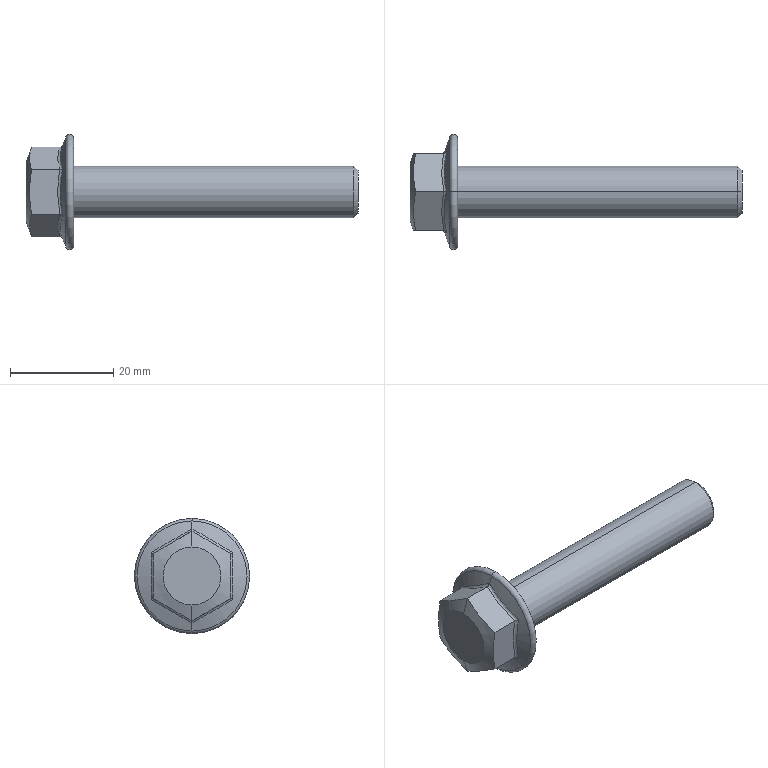Part | SolidWorks | features Fillet 2, RevCut 2, Boss 1, Chamfer 1, Extrusion 1, LPattern 1, Revolution 1 | 1 solid | 25 faces | box 64.2 x 22.3 x 22.3 mm | volume 6417 mm3 | plane 9 | cone 6 | spline 6 | torus 2 | cylinder 2 | commonest cylinder face diameters 10 x2
STEP:
#1=CARTESIAN_POINT('',(64.2,0.,-4.188));
#2=VERTEX_POINT('',#1);
#3=CARTESIAN_POINT('',(64.2,0.,4.188));
#4=VERTEX_POINT('',#3);
#5=CARTESIAN_POINT('',(64.2,0.,0.));
#6=DIRECTION('',(1.,0.,0.));
#7=DIRECTION('',(0.,0.,-1.));
#8=AXIS2_PLACEMENT_3D('',#5,#6,#7);
#9=CIRCLE('',#8,4.188);
#10=EDGE_CURVE('',#2,#4,#9,.T.);
#11=ORIENTED_EDGE('',*,*,#10,.F.);
#12=CARTESIAN_POINT('',(63.388,0.,-5.));
#13=VERTEX_POINT('',#12);
#14=CARTESIAN_POINT('',(64.2,0.,-4.188));
#15=DIRECTION('',(-0.7071,0.,-0.7071));
#16=VECTOR('',#15,1000.);
#17=LINE('',#14,#16);
#18=EDGE_CURVE('',#2,#13,#17,.T.);
#19=ORIENTED_EDGE('',*,*,#18,.T.);
#20=CARTESIAN_POINT('',(63.388,0.,5.));
#21=VERTEX_POINT('',#20);
#22=CARTESIAN_POINT('',(63.388,0.,0.));
#23=DIRECTION('',(-1.,0.,0.));
#24=DIRECTION('',(0.,0.,-1.));
#25=AXIS2_PLACEMENT_3D('',#22,#23,#24);
#26=CIRCLE('',#25,5.);
#27=EDGE_CURVE('',#21,#13,#26,.T.);
#28=ORIENTED_EDGE('',*,*,#27,.F.);
#29=CARTESIAN_POINT('',(64.2,0.,4.188));
#30=DIRECTION('',(-0.7071,0.,0.7071));
#31=VECTOR('',#30,1000.);
#32=LINE('',#29,#31);
#33=EDGE_CURVE('',#4,#21,#32,.T.);
#34=ORIENTED_EDGE('',*,*,#33,.F.);
#35=EDGE_LOOP('',(#11,#19,#28,#34));
#36=FACE_OUTER_BOUND('',#35,.T.);
#37=CARTESIAN_POINT('',(64.2,0.,0.));
#38=DIRECTION('',(-1.,0.,0.));
#39=DIRECTION('',(0.,0.,1.));
#40=AXIS2_PLACEMENT_3D('',#37,#38,#39);
#41=CONICAL_SURFACE('',#40,4.188,0.7854);
#42=ADVANCED_FACE('',(#36),#41,.T.);
#43=CARTESIAN_POINT('',(0.,0.,5.6));
#44=VERTEX_POINT('',#43);
#45=CARTESIAN_POINT('',(0.,0.,-5.6));
#46=VERTEX_POINT('',#45);
#47=CARTESIAN_POINT('',(0.,0.,0.));
#48=DIRECTION('',(-1.,0.,0.));
#49=DIRECTION('',(0.,0.,1.));
#50=AXIS2_PLACEMENT_3D('',#47,#48,#49);
#51=CIRCLE('',#50,5.6);
#52=EDGE_CURVE('',#44,#46,#51,.T.);
#53=ORIENTED_EDGE('',*,*,#52,.F.);
#54=CARTESIAN_POINT('',(1.114,0.,8.66));
#55=VERTEX_POINT('',#54);
#56=CARTESIAN_POINT('',(0.,0.,5.6));
#57=DIRECTION('',(0.342,0.,0.9397));
#58=VECTOR('',#57,1000.);
#59=LINE('',#56,#58);
#60=EDGE_CURVE('',#44,#55,#59,.T.);
#61=ORIENTED_EDGE('',*,*,#60,.T.);
#62=CARTESIAN_POINT('',(1.114,7.5,4.33));
#63=VERTEX_POINT('',#62);
#64=CARTESIAN_POINT('',(1.114,0.,8.66));
#65=CARTESIAN_POINT('',(0.9825,0.625,8.299));
#66=CARTESIAN_POINT('',(0.8759,1.25,7.939));
#67=CARTESIAN_POINT('',(0.7302,2.5,7.217));
#68=CARTESIAN_POINT('',(0.6529,3.75,6.495));
#69=CARTESIAN_POINT('',(0.7302,5.,5.774));
#70=CARTESIAN_POINT('',(0.8759,6.25,5.052));
#71=CARTESIAN_POINT('',(0.9825,6.875,4.691));
#72=CARTESIAN_POINT('',(1.114,7.5,4.33));
#73=B_SPLINE_CURVE_WITH_KNOTS('',3,(#64,#65,#66,#67,#68,#69,#70,#71,#72),.UNSPECIFIED.,.F.,.F.,(4,2,1,2,4),(0.000000231,0.002165,0.00433,0.006495,0.00866),.UNSPECIFIED.);
#74=EDGE_CURVE('',#55,#63,#73,.T.);
#75=ORIENTED_EDGE('',*,*,#74,.T.);
#76=CARTESIAN_POINT('',(1.114,7.5,-4.33));
#77=VERTEX_POINT('',#76);
#78=CARTESIAN_POINT('',(1.114,7.5,4.33));
#79=CARTESIAN_POINT('',(0.983,7.5,3.611));
#80=CARTESIAN_POINT('',(0.8765,7.5,2.891));
#81=CARTESIAN_POINT('',(0.7307,7.5,1.45));
#82=CARTESIAN_POINT('',(0.6918,7.5,0.7288));
#83=CARTESIAN_POINT('',(0.6913,7.5,-0.7155));
#84=CARTESIAN_POINT('',(0.7298,7.5,-1.439));
#85=CARTESIAN_POINT('',(0.8757,7.5,-2.886));
#86=CARTESIAN_POINT('',(0.9832,7.5,-3.612));
#87=CARTESIAN_POINT('',(1.114,7.5,-4.33));
#88=B_SPLINE_CURVE_WITH_KNOTS('',3,(#78,#79,#80,#81,#82,#83,#84,#85,#86,#87),.UNSPECIFIED.,.F.,.F.,(4,2,2,2,4),(0.01595,0.01813,0.02031,0.02249,0.02467),.UNSPECIFIED.);
#89=EDGE_CURVE('',#63,#77,#88,.T.);
#90=ORIENTED_EDGE('',*,*,#89,.T.);
#91=CARTESIAN_POINT('',(1.114,0.,-8.66));
#92=VERTEX_POINT('',#91);
#93=CARTESIAN_POINT('',(1.114,7.5,-4.33));
#94=CARTESIAN_POINT('',(0.9825,6.875,-4.691));
#95=CARTESIAN_POINT('',(0.8759,6.25,-5.052));
#96=CARTESIAN_POINT('',(0.7302,5.,-5.774));
#97=CARTESIAN_POINT('',(0.6529,3.75,-6.495));
#98=CARTESIAN_POINT('',(0.7302,2.5,-7.217));
#99=CARTESIAN_POINT('',(0.8759,1.25,-7.939));
#100=CARTESIAN_POINT('',(0.9825,0.625,-8.299));
#101=CARTESIAN_POINT('',(1.114,0.,-8.66));
#102=B_SPLINE_CURVE_WITH_KNOTS('',3,(#93,#94,#95,#96,#97,#98,#99,#100,#101),.UNSPECIFIED.,.F.,.F.,(4,2,1,2,4),(0.000000231,0.002165,0.00433,0.006495,0.00866),.UNSPECIFIED.);
#103=EDGE_CURVE('',#77,#92,#102,.T.);
#104=ORIENTED_EDGE('',*,*,#103,.T.);
#105=CARTESIAN_POINT('',(0.,0.,-5.6));
#106=DIRECTION('',(0.342,0.,-0.9397));
#107=VECTOR('',#106,1000.);
#108=LINE('',#105,#107);
#109=EDGE_CURVE('',#46,#92,#108,.T.);
#110=ORIENTED_EDGE('',*,*,#109,.F.);
#111=EDGE_LOOP('',(#53,#61,#75,#90,#104,#110));
#112=FACE_OUTER_BOUND('',#111,.T.);
#113=CARTESIAN_POINT('',(0.,0.,0.));
#114=DIRECTION('',(1.,0.,0.));
#115=DIRECTION('',(0.,0.,-1.));
#116=AXIS2_PLACEMENT_3D('',#113,#114,#115);
#117=CONICAL_SURFACE('',#116,5.6,1.222);
#118=ADVANCED_FACE('',(#112),#117,.T.);
#119=CARTESIAN_POINT('',(7.7,0.,-10.641));
#120=VERTEX_POINT('',#119);
#121=CARTESIAN_POINT('',(7.7,0.,10.641));
#122=VERTEX_POINT('',#121);
#123=CARTESIAN_POINT('',(7.7,0.,0.));
#124=DIRECTION('',(1.,0.,0.));
#125=DIRECTION('',(0.,0.,-1.));
#126=AXIS2_PLACEMENT_3D('',#123,#124,#125);
#127=CIRCLE('',#126,10.641);
#128=EDGE_CURVE('',#120,#122,#127,.T.);
#129=ORIENTED_EDGE('',*,*,#128,.T.);
#130=CARTESIAN_POINT('',(9.2,0.,10.377));
#131=VERTEX_POINT('',#130);
#132=CARTESIAN_POINT('',(8.427,0.,10.377));
#133=DIRECTION('',(0.,1.,0.));
#134=DIRECTION('',(0.,0.,1.));
#135=AXIS2_PLACEMENT_3D('',#132,#133,#134);
#136=CIRCLE('',#135,0.7733);
#137=EDGE_CURVE('',#122,#131,#136,.T.);
#138=ORIENTED_EDGE('',*,*,#137,.T.);
#139=CARTESIAN_POINT('',(9.2,0.,-10.377));
#140=VERTEX_POINT('',#139);
#141=CARTESIAN_POINT('',(9.2,0.,0.));
#142=DIRECTION('',(1.,0.,0.));
#143=DIRECTION('',(0.,0.,-1.));
#144=AXIS2_PLACEMENT_3D('',#141,#142,#143);
#145=CIRCLE('',#144,10.377);
#146=EDGE_CURVE('',#140,#131,#145,.T.);
#147=ORIENTED_EDGE('',*,*,#146,.F.);
#148=CARTESIAN_POINT('',(8.427,0.,-10.377));
#149=DIRECTION('',(0.,-1.,0.));
#150=DIRECTION('',(0.,0.,-1.));
#151=AXIS2_PLACEMENT_3D('',#148,#149,#150);
#152=CIRCLE('',#151,0.7733);
#153=EDGE_CURVE('',#120,#140,#152,.T.);
#154=ORIENTED_EDGE('',*,*,#153,.F.);
#155=EDGE_LOOP('',(#129,#138,#147,#154));
#156=FACE_OUTER_BOUND('',#155,.T.);
#157=CARTESIAN_POINT('',(8.427,0.,0.));
#158=DIRECTION('',(1.,0.,0.));
#159=DIRECTION('',(0.,0.,-1.));
#160=AXIS2_PLACEMENT_3D('',#157,#158,#159);
#161=TOROIDAL_SURFACE('',#160,10.377,0.7733);
#162=ADVANCED_FACE('',(#156),#161,.T.);
#163=CARTESIAN_POINT('',(7.156,7.922,4.574));
#164=VERTEX_POINT('',#163);
#165=CARTESIAN_POINT('',(7.156,0.,9.148));
#166=VERTEX_POINT('',#165);
#167=CARTESIAN_POINT('',(7.156,7.922,4.574));
#168=CARTESIAN_POINT('',(7.017,7.265,4.945));
#169=CARTESIAN_POINT('',(6.902,6.605,5.318));
#170=CARTESIAN_POINT('',(6.744,5.282,6.07));
#171=CARTESIAN_POINT('',(6.701,4.619,6.45));
#172=CARTESIAN_POINT('',(6.7,3.287,7.218));
#173=CARTESIAN_POINT('',(6.743,2.624,7.605));
#174=CARTESIAN_POINT('',(6.901,1.305,8.378));
#175=CARTESIAN_POINT('',(7.017,0.6509,8.764));
#176=CARTESIAN_POINT('',(7.156,0.,9.148));
#177=B_SPLINE_CURVE_WITH_KNOTS('',3,(#167,#168,#169,#170,#171,#172,#173,#174,#175,#176),.UNSPECIFIED.,.F.,.F.,(4,2,2,2,4),(0.,0.002295,0.004591,0.006886,0.009181),.UNSPECIFIED.);
#178=EDGE_CURVE('',#164,#166,#177,.T.);
#179=ORIENTED_EDGE('',*,*,#178,.T.);
#180=CARTESIAN_POINT('',(7.7,0.,10.641));
#181=DIRECTION('',(0.342,0.,0.9397));
#182=VECTOR('',#181,1000.);
#183=LINE('',#180,#182);
#184=EDGE_CURVE('',#166,#122,#183,.T.);
#185=ORIENTED_EDGE('',*,*,#184,.T.);
#186=ORIENTED_EDGE('',*,*,#128,.F.);
#187=CARTESIAN_POINT('',(7.156,0.,-9.148));
#188=VERTEX_POINT('',#187);
#189=CARTESIAN_POINT('',(7.7,0.,-10.641));
#190=DIRECTION('',(0.342,0.,-0.9397));
#191=VECTOR('',#190,1000.);
#192=LINE('',#189,#191);
#193=EDGE_CURVE('',#188,#120,#192,.T.);
#194=ORIENTED_EDGE('',*,*,#193,.F.);
#195=CARTESIAN_POINT('',(7.156,7.922,-4.574));
#196=VERTEX_POINT('',#195);
#197=CARTESIAN_POINT('',(7.156,0.,-9.148));
#198=CARTESIAN_POINT('',(7.017,0.6501,-8.764));
#199=CARTESIAN_POINT('',(6.902,1.303,-8.379));
#200=CARTESIAN_POINT('',(6.744,2.616,-7.61));
#201=CARTESIAN_POINT('',(6.701,3.276,-7.225));
#202=CARTESIAN_POINT('',(6.7,4.608,-6.456));
#203=CARTESIAN_POINT('',(6.743,5.274,-6.075));
#204=CARTESIAN_POINT('',(6.901,6.603,-5.319));
#205=CARTESIAN_POINT('',(7.017,7.264,-4.945));
#206=CARTESIAN_POINT('',(7.156,7.922,-4.574));
#207=B_SPLINE_CURVE_WITH_KNOTS('',3,(#197,#198,#199,#200,#201,#202,#203,#204,#205,#206),.UNSPECIFIED.,.F.,.F.,(4,2,2,2,4),(0.,0.002295,0.004591,0.006886,0.009181),.UNSPECIFIED.);
#208=EDGE_CURVE('',#188,#196,#207,.T.);
#209=ORIENTED_EDGE('',*,*,#208,.T.);
#210=CARTESIAN_POINT('',(7.156,7.922,-4.574));
#211=CARTESIAN_POINT('',(7.017,7.915,-3.819));
#212=CARTESIAN_POINT('',(6.902,7.908,-3.062));
#213=CARTESIAN_POINT('',(6.744,7.898,-1.54));
#214=CARTESIAN_POINT('',(6.701,7.895,-0.7751));
#215=CARTESIAN_POINT('',(6.7,7.895,0.7626));
#216=CARTESIAN_POINT('',(6.743,7.898,1.53));
#217=CARTESIAN_POINT('',(6.901,7.908,3.059));
#218=CARTESIAN_POINT('',(7.017,7.915,3.818));
#219=CARTESIAN_POINT('',(7.156,7.922,4.574));
#220=B_SPLINE_CURVE_WITH_KNOTS('',3,(#210,#211,#212,#213,#214,#215,#216,#217,#218,#219),.UNSPECIFIED.,.F.,.F.,(4,2,2,2,4),(0.,0.002295,0.00459,0.006886,0.009181),.UNSPECIFIED.);
#221=EDGE_CURVE('',#196,#164,#220,.T.);
#222=ORIENTED_EDGE('',*,*,#221,.T.);
#223=EDGE_LOOP('',(#179,#185,#186,#194,#209,#222));
#224=FACE_OUTER_BOUND('',#223,.T.);
#225=CARTESIAN_POINT('',(7.7,0.,0.));
#226=DIRECTION('',(1.,0.,0.));
#227=DIRECTION('',(0.,0.,-1.));
#228=AXIS2_PLACEMENT_3D('',#225,#226,#227);
#229=CONICAL_SURFACE('',#228,10.641,1.222);
#230=ADVANCED_FACE('',(#224),#229,.T.);
#231=ORIENTED_EDGE('',*,*,#27,.T.);
#232=CARTESIAN_POINT('',(9.2,0.,-5.));
#233=VERTEX_POINT('',#232);
#234=CARTESIAN_POINT('',(64.2,0.,-5.));
#235=DIRECTION('',(-1.,0.,0.));
#236=VECTOR('',#235,1000.);
#237=LINE('',#234,#236);
#238=EDGE_CURVE('',#13,#233,#237,.T.);
#239=ORIENTED_EDGE('',*,*,#238,.T.);
#240=CARTESIAN_POINT('',(9.2,0.,5.));
#241=VERTEX_POINT('',#240);
#242=CARTESIAN_POINT('',(9.2,0.,0.));
#243=DIRECTION('',(1.,0.,0.));
#244=DIRECTION('',(0.,0.,-1.));
#245=AXIS2_PLACEMENT_3D('',#242,#243,#244);
#246=CIRCLE('',#245,5.);
#247=EDGE_CURVE('',#233,#241,#246,.T.);
#248=ORIENTED_EDGE('',*,*,#247,.T.);
#249=CARTESIAN_POINT('',(64.2,0.,5.));
#250=DIRECTION('',(-1.,0.,0.));
#251=VECTOR('',#250,1000.);
#252=LINE('',#249,#251);
#253=EDGE_CURVE('',#21,#241,#252,.T.);
#254=ORIENTED_EDGE('',*,*,#253,.F.);
#255=EDGE_LOOP('',(#231,#239,#248,#254));
#256=FACE_OUTER_BOUND('',#255,.T.);
#257=CARTESIAN_POINT('',(64.2,0.,0.));
#258=DIRECTION('',(-1.,0.,0.));
#259=DIRECTION('',(0.,0.,1.));
#260=AXIS2_PLACEMENT_3D('',#257,#258,#259);
#261=CYLINDRICAL_SURFACE('',#260,5.);
#262=ADVANCED_FACE('',(#256),#261,.T.);
#263=CARTESIAN_POINT('',(9.2,0.,0.));
#264=DIRECTION('',(1.,0.,0.));
#265=DIRECTION('',(0.,0.,-1.));
#266=AXIS2_PLACEMENT_3D('',#263,#264,#265);
#267=CIRCLE('',#266,5.);
#268=EDGE_CURVE('',#241,#233,#267,.T.);
#269=ORIENTED_EDGE('',*,*,#268,.F.);
#270=ORIENTED_EDGE('',*,*,#247,.F.);
#271=EDGE_LOOP('',(#269,#270));
#272=FACE_BOUND('',#271,.T.);
#273=ORIENTED_EDGE('',*,*,#146,.T.);
#274=CARTESIAN_POINT('',(9.2,0.,0.));
#275=DIRECTION('',(1.,0.,0.));
#276=DIRECTION('',(0.,0.,-1.));
#277=AXIS2_PLACEMENT_3D('',#274,#275,#276);
#278=CIRCLE('',#277,10.377);
#279=EDGE_CURVE('',#131,#140,#278,.T.);
#280=ORIENTED_EDGE('',*,*,#279,.T.);
#281=EDGE_LOOP('',(#273,#280));
#282=FACE_OUTER_BOUND('',#281,.T.);
#283=CARTESIAN_POINT('',(9.2,7.5,-12.99));
#284=DIRECTION('',(1.,0.,0.));
#285=DIRECTION('',(0.,0.,-1.));
#286=AXIS2_PLACEMENT_3D('',#283,#284,#285);
#287=PLANE('',#286);
#288=ADVANCED_FACE('',(#272,#282),#287,.T.);
#289=ORIENTED_EDGE('',*,*,#238,.F.);
#290=CARTESIAN_POINT('',(63.388,0.,0.));
#291=DIRECTION('',(-1.,0.,0.));
#292=DIRECTION('',(0.,0.,-1.));
#293=AXIS2_PLACEMENT_3D('',#290,#291,#292);
#294=CIRCLE('',#293,5.);
#295=EDGE_CURVE('',#13,#21,#294,.T.);
#296=ORIENTED_EDGE('',*,*,#295,.T.);
#297=ORIENTED_EDGE('',*,*,#253,.T.);
#298=ORIENTED_EDGE('',*,*,#268,.T.);
#299=EDGE_LOOP('',(#289,#296,#297,#298));
#300=FACE_OUTER_BOUND('',#299,.T.);
#301=CARTESIAN_POINT('',(64.2,0.,0.));
#302=DIRECTION('',(-1.,0.,0.));
#303=DIRECTION('',(0.,0.,1.));
#304=AXIS2_PLACEMENT_3D('',#301,#302,#303);
#305=CYLINDRICAL_SURFACE('',#304,5.);
#306=ADVANCED_FACE('',(#300),#305,.T.);
#307=CARTESIAN_POINT('',(64.2,0.,0.));
#308=DIRECTION('',(1.,0.,0.));
#309=DIRECTION('',(0.,0.,-1.));
#310=AXIS2_PLACEMENT_3D('',#307,#308,#309);
#311=CIRCLE('',#310,4.188);
#312=EDGE_CURVE('',#4,#2,#311,.T.);
#313=ORIENTED_EDGE('',*,*,#312,.T.);
#314=ORIENTED_EDGE('',*,*,#10,.T.);
#315=EDGE_LOOP('',(#313,#314));
#316=FACE_OUTER_BOUND('',#315,.T.);
#317=CARTESIAN_POINT('',(64.2,0.,0.));
#318=DIRECTION('',(1.,0.,0.));
#319=DIRECTION('',(0.,0.,-1.));
#320=AXIS2_PLACEMENT_3D('',#317,#318,#319);
#321=PLANE('',#320);
#322=ADVANCED_FACE('',(#316),#321,.T.);
#323=ORIENTED_EDGE('',*,*,#184,.F.);
#324=CARTESIAN_POINT('',(7.156,-7.922,4.574));
#325=VERTEX_POINT('',#324);
#326=CARTESIAN_POINT('',(7.156,0.,9.148));
#327=CARTESIAN_POINT('',(7.017,-0.6501,8.764));
#328=CARTESIAN_POINT('',(6.902,-1.303,8.379));
#329=CARTESIAN_POINT('',(6.744,-2.616,7.61));
#330=CARTESIAN_POINT('',(6.701,-3.276,7.225));
#331=CARTESIAN_POINT('',(6.7,-4.608,6.456));
#332=CARTESIAN_POINT('',(6.743,-5.274,6.075));
#333=CARTESIAN_POINT('',(6.901,-6.603,5.319));
#334=CARTESIAN_POINT('',(7.017,-7.264,4.945));
#335=CARTESIAN_POINT('',(7.156,-7.922,4.574));
#336=B_SPLINE_CURVE_WITH_KNOTS('',3,(#326,#327,#328,#329,#330,#331,#332,#333,#334,#335),.UNSPECIFIED.,.F.,.F.,(4,2,2,2,4),(0.,0.002295,0.004591,0.006886,0.009181),.UNSPECIFIED.);
#337=EDGE_CURVE('',#166,#325,#336,.T.);
#338=ORIENTED_EDGE('',*,*,#337,.T.);
#339=CARTESIAN_POINT('',(7.156,-7.922,-4.574));
#340=VERTEX_POINT('',#339);
#341=CARTESIAN_POINT('',(7.156,-7.922,4.574));
#342=CARTESIAN_POINT('',(7.017,-7.915,3.819));
#343=CARTESIAN_POINT('',(6.902,-7.908,3.062));
#344=CARTESIAN_POINT('',(6.744,-7.898,1.54));
#345=CARTESIAN_POINT('',(6.701,-7.895,0.775));
#346=CARTESIAN_POINT('',(6.7,-7.895,-0.7627));
#347=CARTESIAN_POINT('',(6.743,-7.898,-1.53));
#348=CARTESIAN_POINT('',(6.901,-7.908,-3.059));
#349=CARTESIAN_POINT('',(7.017,-7.915,-3.818));
#350=CARTESIAN_POINT('',(7.156,-7.922,-4.574));
#351=B_SPLINE_CURVE_WITH_KNOTS('',3,(#341,#342,#343,#344,#345,#346,#347,#348,#349,#350),.UNSPECIFIED.,.F.,.F.,(4,2,2,2,4),(0.,0.002295,0.004591,0.006886,0.009181),.UNSPECIFIED.);
#352=EDGE_CURVE('',#325,#340,#351,.T.);
#353=ORIENTED_EDGE('',*,*,#352,.T.);
#354=CARTESIAN_POINT('',(7.156,-7.922,-4.574));
#355=CARTESIAN_POINT('',(7.017,-7.265,-4.945));
#356=CARTESIAN_POINT('',(6.902,-6.605,-5.318));
#357=CARTESIAN_POINT('',(6.744,-5.282,-6.07));
#358=CARTESIAN_POINT('',(6.701,-4.619,-6.45));
#359=CARTESIAN_POINT('',(6.7,-3.287,-7.218));
#360=CARTESIAN_POINT('',(6.743,-2.624,-7.605));
#361=CARTESIAN_POINT('',(6.901,-1.305,-8.378));
#362=CARTESIAN_POINT('',(7.017,-0.6509,-8.764));
#363=CARTESIAN_POINT('',(7.156,0.,-9.148));
#364=B_SPLINE_CURVE_WITH_KNOTS('',3,(#354,#355,#356,#357,#358,#359,#360,#361,#362,#363),.UNSPECIFIED.,.F.,.F.,(4,2,2,2,4),(0.,0.002295,0.004591,0.006886,0.009181),.UNSPECIFIED.);
#365=EDGE_CURVE('',#340,#188,#364,.T.);
#366=ORIENTED_EDGE('',*,*,#365,.T.);
#367=ORIENTED_EDGE('',*,*,#193,.T.);
#368=CARTESIAN_POINT('',(7.7,0.,0.));
#369=DIRECTION('',(1.,0.,0.));
#370=DIRECTION('',(0.,0.,-1.));
#371=AXIS2_PLACEMENT_3D('',#368,#369,#370);
#372=CIRCLE('',#371,10.641);
#373=EDGE_CURVE('',#122,#120,#372,.T.);
#374=ORIENTED_EDGE('',*,*,#373,.F.);
#375=EDGE_LOOP('',(#323,#338,#353,#366,#367,#374));
#376=FACE_OUTER_BOUND('',#375,.T.);
#377=CARTESIAN_POINT('',(7.7,0.,0.));
#378=DIRECTION('',(1.,0.,0.));
#379=DIRECTION('',(0.,0.,-1.));
#380=AXIS2_PLACEMENT_3D('',#377,#378,#379);
#381=CONICAL_SURFACE('',#380,10.641,1.222);
#382=ADVANCED_FACE('',(#376),#381,.T.);
#383=ORIENTED_EDGE('',*,*,#137,.F.);
#384=ORIENTED_EDGE('',*,*,#373,.T.);
#385=ORIENTED_EDGE('',*,*,#153,.T.);
#386=ORIENTED_EDGE('',*,*,#279,.F.);
#387=EDGE_LOOP('',(#383,#384,#385,#386));
#388=FACE_OUTER_BOUND('',#387,.T.);
#389=CARTESIAN_POINT('',(8.427,0.,0.));
#390=DIRECTION('',(1.,0.,0.));
#391=DIRECTION('',(0.,0.,-1.));
#392=AXIS2_PLACEMENT_3D('',#389,#390,#391);
#393=TOROIDAL_SURFACE('',#392,10.377,0.7733);
#394=ADVANCED_FACE('',(#388),#393,.T.);
#395=CARTESIAN_POINT('',(0.,0.,0.));
#396=DIRECTION('',(-1.,0.,0.));
#397=DIRECTION('',(0.,0.,1.));
#398=AXIS2_PLACEMENT_3D('',#395,#396,#397);
#399=CIRCLE('',#398,5.6);
#400=EDGE_CURVE('',#46,#44,#399,.T.);
#401=ORIENTED_EDGE('',*,*,#400,.T.);
#402=ORIENTED_EDGE('',*,*,#52,.T.);
#403=EDGE_LOOP('',(#401,#402));
#404=FACE_OUTER_BOUND('',#403,.T.);
#405=CARTESIAN_POINT('',(0.,7.5,-12.99));
#406=DIRECTION('',(1.,0.,0.));
#407=DIRECTION('',(0.,0.,-1.));
#408=AXIS2_PLACEMENT_3D('',#405,#406,#407);
#409=PLANE('',#408);
#410=ADVANCED_FACE('',(#404),#409,.F.);
#411=ORIENTED_EDGE('',*,*,#60,.F.);
#412=ORIENTED_EDGE('',*,*,#400,.F.);
#413=ORIENTED_EDGE('',*,*,#109,.T.);
#414=CARTESIAN_POINT('',(1.114,-7.5,-4.33));
#415=VERTEX_POINT('',#414);
#416=CARTESIAN_POINT('',(1.114,0.,-8.66));
#417=CARTESIAN_POINT('',(0.9825,-0.625,-8.299));
#418=CARTESIAN_POINT('',(0.8759,-1.25,-7.939));
#419=CARTESIAN_POINT('',(0.7302,-2.5,-7.217));
#420=CARTESIAN_POINT('',(0.6529,-3.75,-6.495));
#421=CARTESIAN_POINT('',(0.7302,-5.,-5.774));
#422=CARTESIAN_POINT('',(0.8759,-6.25,-5.052));
#423=CARTESIAN_POINT('',(0.9825,-6.875,-4.691));
#424=CARTESIAN_POINT('',(1.114,-7.5,-4.33));
#425=B_SPLINE_CURVE_WITH_KNOTS('',3,(#416,#417,#418,#419,#420,#421,#422,#423,#424),.UNSPECIFIED.,.F.,.F.,(4,2,1,2,4),(0.000000231,0.002165,0.00433,0.006495,0.00866),.UNSPECIFIED.);
#426=EDGE_CURVE('',#92,#415,#425,.T.);
#427=ORIENTED_EDGE('',*,*,#426,.T.);
#428=CARTESIAN_POINT('',(1.114,-7.5,4.33));
#429=VERTEX_POINT('',#428);
#430=CARTESIAN_POINT('',(1.114,-7.5,-4.33));
#431=CARTESIAN_POINT('',(0.9832,-7.5,-3.612));
#432=CARTESIAN_POINT('',(0.8757,-7.5,-2.886));
#433=CARTESIAN_POINT('',(0.7298,-7.5,-1.439));
#434=CARTESIAN_POINT('',(0.6913,-7.5,-0.7155));
#435=CARTESIAN_POINT('',(0.6918,-7.5,0.7288));
#436=CARTESIAN_POINT('',(0.7307,-7.5,1.45));
#437=CARTESIAN_POINT('',(0.8765,-7.5,2.891));
#438=CARTESIAN_POINT('',(0.983,-7.5,3.611));
#439=CARTESIAN_POINT('',(1.114,-7.5,4.33));
#440=B_SPLINE_CURVE_WITH_KNOTS('',3,(#430,#431,#432,#433,#434,#435,#436,#437,#438,#439),.UNSPECIFIED.,.F.,.F.,(4,2,2,2,4),(0.007297,0.009483,0.01167,0.01385,0.01604),.UNSPECIFIED.);
#441=EDGE_CURVE('',#415,#429,#440,.T.);
#442=ORIENTED_EDGE('',*,*,#441,.T.);
#443=CARTESIAN_POINT('',(1.114,-7.5,4.33));
#444=CARTESIAN_POINT('',(0.9825,-6.875,4.691));
#445=CARTESIAN_POINT('',(0.8759,-6.25,5.052));
#446=CARTESIAN_POINT('',(0.7302,-5.,5.774));
#447=CARTESIAN_POINT('',(0.6529,-3.75,6.495));
#448=CARTESIAN_POINT('',(0.7302,-2.5,7.217));
#449=CARTESIAN_POINT('',(0.8759,-1.25,7.939));
#450=CARTESIAN_POINT('',(0.9825,-0.625,8.299));
#451=CARTESIAN_POINT('',(1.114,0.,8.66));
#452=B_SPLINE_CURVE_WITH_KNOTS('',3,(#443,#444,#445,#446,#447,#448,#449,#450,#451),.UNSPECIFIED.,.F.,.F.,(4,2,1,2,4),(0.000000231,0.002165,0.00433,0.006495,0.00866),.UNSPECIFIED.);
#453=EDGE_CURVE('',#429,#55,#452,.T.);
#454=ORIENTED_EDGE('',*,*,#453,.T.);
#455=EDGE_LOOP('',(#411,#412,#413,#427,#442,#454));
#456=FACE_OUTER_BOUND('',#455,.T.);
#457=CARTESIAN_POINT('',(0.,0.,0.));
#458=DIRECTION('',(1.,0.,0.));
#459=DIRECTION('',(0.,0.,-1.));
#460=AXIS2_PLACEMENT_3D('',#457,#458,#459);
#461=CONICAL_SURFACE('',#460,5.6,1.222);
#462=ADVANCED_FACE('',(#456),#461,.T.);
#463=CARTESIAN_POINT('',(6.531,-7.5,-4.33));
#464=VERTEX_POINT('',#463);
#465=CARTESIAN_POINT('',(9.2,-7.5,-4.33));
#466=DIRECTION('',(-1.,0.,0.));
#467=VECTOR('',#466,1000.);
#468=LINE('',#465,#467);
#469=EDGE_CURVE('',#464,#415,#468,.T.);
#470=ORIENTED_EDGE('',*,*,#469,.F.);
#471=CARTESIAN_POINT('',(6.531,-7.5,4.33));
#472=VERTEX_POINT('',#471);
#473=CARTESIAN_POINT('',(6.531,-7.5,-4.33));
#474=CARTESIAN_POINT('',(6.286,-7.5,-2.897));
#475=CARTESIAN_POINT('',(6.137,-7.5,-1.455));
#476=CARTESIAN_POINT('',(6.137,-7.5,1.455));
#477=CARTESIAN_POINT('',(6.286,-7.5,2.897));
#478=CARTESIAN_POINT('',(6.531,-7.5,4.33));
#479=B_SPLINE_CURVE_WITH_KNOTS('',3,(#473,#474,#475,#476,#477,#478),.UNSPECIFIED.,.F.,.F.,(4,2,4),(0.,0.004348,0.008696),.UNSPECIFIED.);
#480=EDGE_CURVE('',#464,#472,#479,.T.);
#481=ORIENTED_EDGE('',*,*,#480,.T.);
#482=CARTESIAN_POINT('',(9.2,-7.5,4.33));
#483=DIRECTION('',(-1.,0.,0.));
#484=VECTOR('',#483,1000.);
#485=LINE('',#482,#484);
#486=EDGE_CURVE('',#472,#429,#485,.T.);
#487=ORIENTED_EDGE('',*,*,#486,.T.);
#488=ORIENTED_EDGE('',*,*,#441,.F.);
#489=EDGE_LOOP('',(#470,#481,#487,#488));
#490=FACE_OUTER_BOUND('',#489,.T.);
#491=CARTESIAN_POINT('',(9.2,-7.5,4.33));
#492=DIRECTION('',(0.,1.,0.));
#493=DIRECTION('',(0.,0.,1.));
#494=AXIS2_PLACEMENT_3D('',#491,#492,#493);
#495=PLANE('',#494);
#496=ADVANCED_FACE('',(#490),#495,.F.);
#497=ORIENTED_EDGE('',*,*,#486,.F.);
#498=CARTESIAN_POINT('',(6.531,0.,8.66));
#499=VERTEX_POINT('',#498);
#500=CARTESIAN_POINT('',(6.531,-7.5,4.33));
#501=CARTESIAN_POINT('',(6.286,-6.259,5.047));
#502=CARTESIAN_POINT('',(6.137,-5.01,5.768));
#503=CARTESIAN_POINT('',(6.137,-2.49,7.223));
#504=CARTESIAN_POINT('',(6.286,-1.241,7.944));
#505=CARTESIAN_POINT('',(6.531,0.,8.66));
#506=B_SPLINE_CURVE_WITH_KNOTS('',3,(#500,#501,#502,#503,#504,#505),.UNSPECIFIED.,.F.,.F.,(4,2,4),(0.,0.004348,0.008696),.UNSPECIFIED.);
#507=EDGE_CURVE('',#472,#499,#506,.T.);
#508=ORIENTED_EDGE('',*,*,#507,.T.);
#509=CARTESIAN_POINT('',(9.2,0.,8.66));
#510=DIRECTION('',(-1.,0.,0.));
#511=VECTOR('',#510,1000.);
#512=LINE('',#509,#511);
#513=EDGE_CURVE('',#499,#55,#512,.T.);
#514=ORIENTED_EDGE('',*,*,#513,.T.);
#515=ORIENTED_EDGE('',*,*,#453,.F.);
#516=EDGE_LOOP('',(#497,#508,#514,#515));
#517=FACE_OUTER_BOUND('',#516,.T.);
#518=CARTESIAN_POINT('',(9.2,0.,8.66));
#519=DIRECTION('',(0.,0.5,-0.866));
#520=DIRECTION('',(0.,0.866,0.5));
#521=AXIS2_PLACEMENT_3D('',#518,#519,#520);
#522=PLANE('',#521);
#523=ADVANCED_FACE('',(#517),#522,.F.);
#524=ORIENTED_EDGE('',*,*,#513,.F.);
#525=CARTESIAN_POINT('',(6.531,7.5,4.33));
#526=VERTEX_POINT('',#525);
#527=CARTESIAN_POINT('',(6.531,0.,8.66));
#528=CARTESIAN_POINT('',(6.286,1.241,7.944));
#529=CARTESIAN_POINT('',(6.137,2.49,7.223));
#530=CARTESIAN_POINT('',(6.137,5.01,5.768));
#531=CARTESIAN_POINT('',(6.286,6.259,5.047));
#532=CARTESIAN_POINT('',(6.531,7.5,4.33));
#533=B_SPLINE_CURVE_WITH_KNOTS('',3,(#527,#528,#529,#530,#531,#532),.UNSPECIFIED.,.F.,.F.,(4,2,4),(0.,0.004348,0.008696),.UNSPECIFIED.);
#534=EDGE_CURVE('',#499,#526,#533,.T.);
#535=ORIENTED_EDGE('',*,*,#534,.T.);
#536=CARTESIAN_POINT('',(9.2,7.5,4.33));
#537=DIRECTION('',(-1.,0.,0.));
#538=VECTOR('',#537,1000.);
#539=LINE('',#536,#538);
#540=EDGE_CURVE('',#526,#63,#539,.T.);
#541=ORIENTED_EDGE('',*,*,#540,.T.);
#542=ORIENTED_EDGE('',*,*,#74,.F.);
#543=EDGE_LOOP('',(#524,#535,#541,#542));
#544=FACE_OUTER_BOUND('',#543,.T.);
#545=CARTESIAN_POINT('',(9.2,7.5,4.33));
#546=DIRECTION('',(0.,-0.5,-0.866));
#547=DIRECTION('',(0.,0.866,-0.5));
#548=AXIS2_PLACEMENT_3D('',#545,#546,#547);
#549=PLANE('',#548);
#550=ADVANCED_FACE('',(#544),#549,.F.);
#551=ORIENTED_EDGE('',*,*,#540,.F.);
#552=CARTESIAN_POINT('',(6.531,7.5,-4.33));
#553=VERTEX_POINT('',#552);
#554=CARTESIAN_POINT('',(6.531,7.5,4.33));
#555=CARTESIAN_POINT('',(6.286,7.5,2.897));
#556=CARTESIAN_POINT('',(6.137,7.5,1.455));
#557=CARTESIAN_POINT('',(6.137,7.5,-1.455));
#558=CARTESIAN_POINT('',(6.286,7.5,-2.897));
#559=CARTESIAN_POINT('',(6.531,7.5,-4.33));
#560=B_SPLINE_CURVE_WITH_KNOTS('',3,(#554,#555,#556,#557,#558,#559),.UNSPECIFIED.,.F.,.F.,(4,2,4),(0.,0.004348,0.008696),.UNSPECIFIED.);
#561=EDGE_CURVE('',#526,#553,#560,.T.);
#562=ORIENTED_EDGE('',*,*,#561,.T.);
#563=CARTESIAN_POINT('',(9.2,7.5,-4.33));
#564=DIRECTION('',(-1.,0.,0.));
#565=VECTOR('',#564,1000.);
#566=LINE('',#563,#565);
#567=EDGE_CURVE('',#553,#77,#566,.T.);
#568=ORIENTED_EDGE('',*,*,#567,.T.);
#569=ORIENTED_EDGE('',*,*,#89,.F.);
#570=EDGE_LOOP('',(#551,#562,#568,#569));
#571=FACE_OUTER_BOUND('',#570,.T.);
#572=CARTESIAN_POINT('',(9.2,7.5,-4.33));
#573=DIRECTION('',(0.,-1.,0.));
#574=DIRECTION('',(0.,0.,-1.));
#575=AXIS2_PLACEMENT_3D('',#572,#573,#574);
#576=PLANE('',#575);
#577=ADVANCED_FACE('',(#571),#576,.F.);
#578=ORIENTED_EDGE('',*,*,#567,.F.);
#579=CARTESIAN_POINT('',(6.531,0.,-8.66));
#580=VERTEX_POINT('',#579);
#581=CARTESIAN_POINT('',(6.531,7.5,-4.33));
#582=CARTESIAN_POINT('',(6.286,6.259,-5.047));
#583=CARTESIAN_POINT('',(6.137,5.01,-5.768));
#584=CARTESIAN_POINT('',(6.137,2.49,-7.223));
#585=CARTESIAN_POINT('',(6.286,1.241,-7.944));
#586=CARTESIAN_POINT('',(6.531,0.,-8.66));
#587=B_SPLINE_CURVE_WITH_KNOTS('',3,(#581,#582,#583,#584,#585,#586),.UNSPECIFIED.,.F.,.F.,(4,2,4),(0.,0.004348,0.008696),.UNSPECIFIED.);
#588=EDGE_CURVE('',#553,#580,#587,.T.);
#589=ORIENTED_EDGE('',*,*,#588,.T.);
#590=CARTESIAN_POINT('',(9.2,0.,-8.66));
#591=DIRECTION('',(-1.,0.,0.));
#592=VECTOR('',#591,1000.);
#593=LINE('',#590,#592);
#594=EDGE_CURVE('',#580,#92,#593,.T.);
#595=ORIENTED_EDGE('',*,*,#594,.T.);
#596=ORIENTED_EDGE('',*,*,#103,.F.);
#597=EDGE_LOOP('',(#578,#589,#595,#596));
#598=FACE_OUTER_BOUND('',#597,.T.);
#599=CARTESIAN_POINT('',(9.2,0.,-8.66));
#600=DIRECTION('',(0.,-0.5,0.866));
#601=DIRECTION('',(0.,-0.866,-0.5));
#602=AXIS2_PLACEMENT_3D('',#599,#600,#601);
#603=PLANE('',#602);
#604=ADVANCED_FACE('',(#598),#603,.F.);
#605=ORIENTED_EDGE('',*,*,#594,.F.);
#606=CARTESIAN_POINT('',(6.531,0.,-8.66));
#607=CARTESIAN_POINT('',(6.286,-1.241,-7.944));
#608=CARTESIAN_POINT('',(6.137,-2.49,-7.223));
#609=CARTESIAN_POINT('',(6.137,-5.01,-5.768));
#610=CARTESIAN_POINT('',(6.286,-6.259,-5.047));
#611=CARTESIAN_POINT('',(6.531,-7.5,-4.33));
#612=B_SPLINE_CURVE_WITH_KNOTS('',3,(#606,#607,#608,#609,#610,#611),.UNSPECIFIED.,.F.,.F.,(4,2,4),(0.,0.004348,0.008696),.UNSPECIFIED.);
#613=EDGE_CURVE('',#580,#464,#612,.T.);
#614=ORIENTED_EDGE('',*,*,#613,.T.);
#615=ORIENTED_EDGE('',*,*,#469,.T.);
#616=ORIENTED_EDGE('',*,*,#426,.F.);
#617=EDGE_LOOP('',(#605,#614,#615,#616));
#618=FACE_OUTER_BOUND('',#617,.T.);
#619=CARTESIAN_POINT('',(9.2,-7.5,-4.33));
#620=DIRECTION('',(0.,0.5,0.866));
#621=DIRECTION('',(0.,-0.866,0.5));
#622=AXIS2_PLACEMENT_3D('',#619,#620,#621);
#623=PLANE('',#622);
#624=ADVANCED_FACE('',(#618),#623,.F.);
#625=CARTESIAN_POINT('',(7.156,0.,-9.148));
#626=CARTESIAN_POINT('',(7.109,0.,-9.016));
#627=CARTESIAN_POINT('',(7.027,0.,-8.896));
#628=CARTESIAN_POINT('',(6.809,0.,-8.717));
#629=CARTESIAN_POINT('',(6.673,0.,-8.66));
#630=CARTESIAN_POINT('',(6.531,0.,-8.66));
#631=B_SPLINE_CURVE_WITH_KNOTS('',3,(#625,#626,#627,#628,#629,#630),.UNSPECIFIED.,.F.,.F.,(4,2,4),(-0.000005145,0.0004153,0.0008358),.UNSPECIFIED.);
#632=EDGE_CURVE('',#188,#580,#631,.T.);
#633=ORIENTED_EDGE('',*,*,#632,.F.);
#634=ORIENTED_EDGE('',*,*,#365,.F.);
#635=CARTESIAN_POINT('',(6.531,-7.5,-4.33));
#636=CARTESIAN_POINT('',(6.673,-7.5,-4.33));
#637=CARTESIAN_POINT('',(6.809,-7.549,-4.358));
#638=CARTESIAN_POINT('',(7.027,-7.704,-4.448));
#639=CARTESIAN_POINT('',(7.109,-7.809,-4.508));
#640=CARTESIAN_POINT('',(7.156,-7.922,-4.574));
#641=B_SPLINE_CURVE_WITH_KNOTS('',3,(#635,#636,#637,#638,#639,#640),.UNSPECIFIED.,.F.,.F.,(4,2,4),(0.,0.000419,0.000838),.UNSPECIFIED.);
#642=EDGE_CURVE('',#464,#340,#641,.T.);
#643=ORIENTED_EDGE('',*,*,#642,.F.);
#644=ORIENTED_EDGE('',*,*,#613,.F.);
#645=EDGE_LOOP('',(#633,#634,#643,#644));
#646=FACE_OUTER_BOUND('',#645,.T.);
#647=CARTESIAN_POINT('',(6.603,0.3471,-8.861));
#648=CARTESIAN_POINT('',(7.038,0.2779,-8.821));
#649=CARTESIAN_POINT('',(7.166,0.04606,-9.175));
#650=CARTESIAN_POINT('',(6.322,-0.9764,-8.097));
#651=CARTESIAN_POINT('',(6.752,-1.016,-8.074));
#652=CARTESIAN_POINT('',(6.886,-1.249,-8.41));
#653=CARTESIAN_POINT('',(6.139,-2.325,-7.318));
#654=CARTESIAN_POINT('',(6.559,-2.352,-7.302));
#655=CARTESIAN_POINT('',(6.703,-2.559,-7.639));
#656=CARTESIAN_POINT('',(6.135,-4.419,-6.109));
#657=CARTESIAN_POINT('',(6.555,-4.406,-6.116));
#658=CARTESIAN_POINT('',(6.699,-4.599,-6.46));
#659=CARTESIAN_POINT('',(6.179,-5.112,-5.709));
#660=CARTESIAN_POINT('',(6.601,-5.089,-5.722));
#661=CARTESIAN_POINT('',(6.743,-5.276,-6.073));
#662=CARTESIAN_POINT('',(6.341,-6.487,-4.915));
#663=CARTESIAN_POINT('',(6.768,-6.44,-4.942));
#664=CARTESIAN_POINT('',(6.905,-6.626,-5.306));
#665=CARTESIAN_POINT('',(6.459,-7.169,-4.521));
#666=CARTESIAN_POINT('',(6.891,-7.112,-4.554));
#667=CARTESIAN_POINT('',(7.023,-7.298,-4.926));
#668=CARTESIAN_POINT('',(6.603,-7.848,-4.129));
#669=CARTESIAN_POINT('',(7.038,-7.779,-4.169));
#670=CARTESIAN_POINT('',(7.167,-7.97,-4.547));
#671=(BOUNDED_SURFACE()B_SPLINE_SURFACE(3,2,((#647,#648,#649),(#650,#651,#652),(#653,#654,#655),(#656,#657,#658),(#659,#660,#661),(#662,#663,#664),(#665,#666,#667),(#668,#669,#670)),.UNSPECIFIED.,.F.,.F.,.F.)B_SPLINE_SURFACE_WITH_KNOTS((4,2,2,4),(3,3),(0.03879,0.04342,0.04574,0.04806),(0.,1.),.UNSPECIFIED.)GEOMETRIC_REPRESENTATION_ITEM()RATIONAL_B_SPLINE_SURFACE(((1.,0.8048,1.),(1.,0.8124,1.),(1.,0.8191,1.),(1.,0.8192,1.),(1.,0.8176,1.),(1.,0.8123,1.),(1.,0.8086,1.),(1.,0.8048,1.)))REPRESENTATION_ITEM('')SURFACE());
#672=ADVANCED_FACE('',(#646),#671,.F.);
#673=ORIENTED_EDGE('',*,*,#642,.T.);
#674=ORIENTED_EDGE('',*,*,#352,.F.);
#675=CARTESIAN_POINT('',(6.531,-7.5,4.33));
#676=CARTESIAN_POINT('',(6.673,-7.5,4.33));
#677=CARTESIAN_POINT('',(6.809,-7.549,4.358));
#678=CARTESIAN_POINT('',(7.027,-7.704,4.448));
#679=CARTESIAN_POINT('',(7.109,-7.809,4.508));
#680=CARTESIAN_POINT('',(7.156,-7.922,4.574));
#681=B_SPLINE_CURVE_WITH_KNOTS('',3,(#675,#676,#677,#678,#679,#680),.UNSPECIFIED.,.F.,.F.,(4,2,4),(0.,0.000419,0.000838),.UNSPECIFIED.);
#682=EDGE_CURVE('',#472,#325,#681,.T.);
#683=ORIENTED_EDGE('',*,*,#682,.F.);
#684=ORIENTED_EDGE('',*,*,#480,.F.);
#685=EDGE_LOOP('',(#673,#674,#683,#684));
#686=FACE_OUTER_BOUND('',#685,.T.);
#687=CARTESIAN_POINT('',(6.603,-7.5,-4.731));
#688=CARTESIAN_POINT('',(7.038,-7.5,-4.651));
#689=CARTESIAN_POINT('',(7.166,-7.923,-4.627));
#690=CARTESIAN_POINT('',(6.322,-7.5,-3.203));
#691=CARTESIAN_POINT('',(6.752,-7.5,-3.157));
#692=CARTESIAN_POINT('',(6.886,-7.908,-3.123));
#693=CARTESIAN_POINT('',(6.139,-7.5,-1.645));
#694=CARTESIAN_POINT('',(6.559,-7.5,-1.614));
#695=CARTESIAN_POINT('',(6.703,-7.895,-1.603));
#696=CARTESIAN_POINT('',(6.135,-7.5,0.7723));
#697=CARTESIAN_POINT('',(6.555,-7.5,0.7577));
#698=CARTESIAN_POINT('',(6.699,-7.895,0.7528));
#699=CARTESIAN_POINT('',(6.179,-7.5,1.573));
#700=CARTESIAN_POINT('',(6.601,-7.5,1.545));
#701=CARTESIAN_POINT('',(6.743,-7.898,1.533));
#702=CARTESIAN_POINT('',(6.341,-7.5,3.16));
#703=CARTESIAN_POINT('',(6.768,-7.5,3.106));
#704=CARTESIAN_POINT('',(6.905,-7.908,3.085));
#705=CARTESIAN_POINT('',(6.459,-7.5,3.948));
#706=CARTESIAN_POINT('',(6.891,-7.5,3.883));
#707=CARTESIAN_POINT('',(7.023,-7.915,3.857));
#708=CARTESIAN_POINT('',(6.603,-7.5,4.732));
#709=CARTESIAN_POINT('',(7.038,-7.5,4.652));
#710=CARTESIAN_POINT('',(7.167,-7.923,4.629));
#711=(BOUNDED_SURFACE()B_SPLINE_SURFACE(3,2,((#687,#688,#689),(#690,#691,#692),(#693,#694,#695),(#696,#697,#698),(#699,#700,#701),(#702,#703,#704),(#705,#706,#707),(#708,#709,#710)),.UNSPECIFIED.,.F.,.F.,.F.)B_SPLINE_SURFACE_WITH_KNOTS((4,2,2,4),(3,3),(0.03869,0.04332,0.04564,0.04796),(0.,1.),.UNSPECIFIED.)GEOMETRIC_REPRESENTATION_ITEM()RATIONAL_B_SPLINE_SURFACE(((1.,0.8048,1.),(1.,0.8124,1.),(1.,0.8191,1.),(1.,0.8192,1.),(1.,0.8176,1.),(1.,0.8123,1.),(1.,0.8086,1.),(1.,0.8048,1.)))REPRESENTATION_ITEM('')SURFACE());
#712=ADVANCED_FACE('',(#686),#711,.F.);
#713=ORIENTED_EDGE('',*,*,#632,.T.);
#714=ORIENTED_EDGE('',*,*,#588,.F.);
#715=CARTESIAN_POINT('',(7.156,7.922,-4.574));
#716=CARTESIAN_POINT('',(7.109,7.808,-4.508));
#717=CARTESIAN_POINT('',(7.027,7.704,-4.448));
#718=CARTESIAN_POINT('',(6.809,7.549,-4.358));
#719=CARTESIAN_POINT('',(6.673,7.5,-4.33));
#720=CARTESIAN_POINT('',(6.531,7.5,-4.33));
#721=B_SPLINE_CURVE_WITH_KNOTS('',3,(#715,#716,#717,#718,#719,#720),.UNSPECIFIED.,.F.,.F.,(4,2,4),(-0.000005145,0.0004153,0.0008358),.UNSPECIFIED.);
#722=EDGE_CURVE('',#196,#553,#721,.T.);
#723=ORIENTED_EDGE('',*,*,#722,.F.);
#724=ORIENTED_EDGE('',*,*,#208,.F.);
#725=EDGE_LOOP('',(#713,#714,#723,#724));
#726=FACE_OUTER_BOUND('',#725,.T.);
#727=CARTESIAN_POINT('',(6.603,7.847,-4.13));
#728=CARTESIAN_POINT('',(7.038,7.778,-4.17));
#729=CARTESIAN_POINT('',(7.166,7.969,-4.548));
#730=CARTESIAN_POINT('',(6.322,6.524,-4.894));
#731=CARTESIAN_POINT('',(6.752,6.484,-4.917));
#732=CARTESIAN_POINT('',(6.886,6.659,-5.287));
#733=CARTESIAN_POINT('',(6.139,5.175,-5.673));
#734=CARTESIAN_POINT('',(6.559,5.148,-5.688));
#735=CARTESIAN_POINT('',(6.703,5.336,-6.036));
#736=CARTESIAN_POINT('',(6.135,3.081,-6.881));
#737=CARTESIAN_POINT('',(6.555,3.094,-6.874));
#738=CARTESIAN_POINT('',(6.699,3.295,-7.214));
#739=CARTESIAN_POINT('',(6.179,2.388,-7.282));
#740=CARTESIAN_POINT('',(6.601,2.411,-7.268));
#741=CARTESIAN_POINT('',(6.743,2.621,-7.606));
#742=CARTESIAN_POINT('',(6.341,1.013,-8.075));
#743=CARTESIAN_POINT('',(6.768,1.06,-8.048));
#744=CARTESIAN_POINT('',(6.905,1.283,-8.391));
#745=CARTESIAN_POINT('',(6.459,0.3307,-8.469));
#746=CARTESIAN_POINT('',(6.891,0.3875,-8.437));
#747=CARTESIAN_POINT('',(7.023,0.617,-8.784));
#748=CARTESIAN_POINT('',(6.603,-0.3483,-8.861));
#749=CARTESIAN_POINT('',(7.038,-0.2791,-8.821));
#750=CARTESIAN_POINT('',(7.167,-0.04726,-9.176));
#751=(BOUNDED_SURFACE()B_SPLINE_SURFACE(3,2,((#727,#728,#729),(#730,#731,#732),(#733,#734,#735),(#736,#737,#738),(#739,#740,#741),(#742,#743,#744),(#745,#746,#747),(#748,#749,#750)),.UNSPECIFIED.,.F.,.F.,.F.)B_SPLINE_SURFACE_WITH_KNOTS((4,2,2,4),(3,3),(0.03879,0.04342,0.04574,0.04806),(0.,1.),.UNSPECIFIED.)GEOMETRIC_REPRESENTATION_ITEM()RATIONAL_B_SPLINE_SURFACE(((1.,0.8048,1.),(1.,0.8124,1.),(1.,0.8191,1.),(1.,0.8192,1.),(1.,0.8176,1.),(1.,0.8123,1.),(1.,0.8086,1.),(1.,0.8048,1.)))REPRESENTATION_ITEM('')SURFACE());
#752=ADVANCED_FACE('',(#726),#751,.F.);
#753=ORIENTED_EDGE('',*,*,#682,.T.);
#754=ORIENTED_EDGE('',*,*,#337,.F.);
#755=CARTESIAN_POINT('',(6.531,0.,8.66));
#756=CARTESIAN_POINT('',(6.673,0.,8.66));
#757=CARTESIAN_POINT('',(6.809,0.,8.717));
#758=CARTESIAN_POINT('',(7.027,0.,8.896));
#759=CARTESIAN_POINT('',(7.109,0.,9.017));
#760=CARTESIAN_POINT('',(7.156,0.,9.148));
#761=B_SPLINE_CURVE_WITH_KNOTS('',3,(#755,#756,#757,#758,#759,#760),.UNSPECIFIED.,.F.,.F.,(4,2,4),(0.,0.000419,0.000838),.UNSPECIFIED.);
#762=EDGE_CURVE('',#499,#166,#761,.T.);
#763=ORIENTED_EDGE('',*,*,#762,.F.);
#764=ORIENTED_EDGE('',*,*,#507,.F.);
#765=EDGE_LOOP('',(#753,#754,#763,#764));
#766=FACE_OUTER_BOUND('',#765,.T.);
#767=CARTESIAN_POINT('',(6.603,-7.847,4.13));
#768=CARTESIAN_POINT('',(7.038,-7.778,4.17));
#769=CARTESIAN_POINT('',(7.166,-7.969,4.548));
#770=CARTESIAN_POINT('',(6.322,-6.524,4.894));
#771=CARTESIAN_POINT('',(6.752,-6.484,4.917));
#772=CARTESIAN_POINT('',(6.886,-6.659,5.287));
#773=CARTESIAN_POINT('',(6.139,-5.175,5.673));
#774=CARTESIAN_POINT('',(6.559,-5.148,5.688));
#775=CARTESIAN_POINT('',(6.703,-5.336,6.036));
#776=CARTESIAN_POINT('',(6.135,-3.081,6.881));
#777=CARTESIAN_POINT('',(6.555,-3.094,6.874));
#778=CARTESIAN_POINT('',(6.699,-3.295,7.214));
#779=CARTESIAN_POINT('',(6.179,-2.388,7.282));
#780=CARTESIAN_POINT('',(6.601,-2.411,7.268));
#781=CARTESIAN_POINT('',(6.743,-2.621,7.606));
#782=CARTESIAN_POINT('',(6.341,-1.013,8.075));
#783=CARTESIAN_POINT('',(6.768,-1.06,8.048));
#784=CARTESIAN_POINT('',(6.905,-1.283,8.391));
#785=CARTESIAN_POINT('',(6.459,-0.3307,8.469));
#786=CARTESIAN_POINT('',(6.891,-0.3875,8.437));
#787=CARTESIAN_POINT('',(7.023,-0.617,8.784));
#788=CARTESIAN_POINT('',(6.603,0.3483,8.861));
#789=CARTESIAN_POINT('',(7.038,0.2791,8.821));
#790=CARTESIAN_POINT('',(7.167,0.04726,9.176));
#791=(BOUNDED_SURFACE()B_SPLINE_SURFACE(3,2,((#767,#768,#769),(#770,#771,#772),(#773,#774,#775),(#776,#777,#778),(#779,#780,#781),(#782,#783,#784),(#785,#786,#787),(#788,#789,#790)),.UNSPECIFIED.,.F.,.F.,.T.)B_SPLINE_SURFACE_WITH_KNOTS((4,2,2,4),(3,3),(0.03879,0.04342,0.04574,0.04806),(0.,1.),.UNSPECIFIED.)GEOMETRIC_REPRESENTATION_ITEM()RATIONAL_B_SPLINE_SURFACE(((1.,0.8048,1.),(1.,0.8124,1.),(1.,0.8191,1.),(1.,0.8192,1.),(1.,0.8176,1.),(1.,0.8123,1.),(1.,0.8086,1.),(1.,0.8048,1.)))REPRESENTATION_ITEM('')SURFACE());
#792=ADVANCED_FACE('',(#766),#791,.F.);
#793=ORIENTED_EDGE('',*,*,#722,.T.);
#794=ORIENTED_EDGE('',*,*,#561,.F.);
#795=CARTESIAN_POINT('',(7.156,7.922,4.574));
#796=CARTESIAN_POINT('',(7.109,7.808,4.508));
#797=CARTESIAN_POINT('',(7.027,7.704,4.448));
#798=CARTESIAN_POINT('',(6.809,7.549,4.358));
#799=CARTESIAN_POINT('',(6.673,7.5,4.33));
#800=CARTESIAN_POINT('',(6.531,7.5,4.33));
#801=B_SPLINE_CURVE_WITH_KNOTS('',3,(#795,#796,#797,#798,#799,#800),.UNSPECIFIED.,.F.,.F.,(4,2,4),(-0.000005145,0.0004153,0.0008358),.UNSPECIFIED.);
#802=EDGE_CURVE('',#164,#526,#801,.T.);
#803=ORIENTED_EDGE('',*,*,#802,.F.);
#804=ORIENTED_EDGE('',*,*,#221,.F.);
#805=EDGE_LOOP('',(#793,#794,#803,#804));
#806=FACE_OUTER_BOUND('',#805,.T.);
#807=CARTESIAN_POINT('',(6.603,7.5,4.731));
#808=CARTESIAN_POINT('',(7.038,7.5,4.651));
#809=CARTESIAN_POINT('',(7.166,7.923,4.627));
#810=CARTESIAN_POINT('',(6.322,7.5,3.203));
#811=CARTESIAN_POINT('',(6.752,7.5,3.157));
#812=CARTESIAN_POINT('',(6.886,7.908,3.123));
#813=CARTESIAN_POINT('',(6.139,7.5,1.645));
#814=CARTESIAN_POINT('',(6.559,7.5,1.614));
#815=CARTESIAN_POINT('',(6.703,7.895,1.603));
#816=CARTESIAN_POINT('',(6.135,7.5,-0.7729));
#817=CARTESIAN_POINT('',(6.555,7.5,-0.7583));
#818=CARTESIAN_POINT('',(6.699,7.895,-0.7534));
#819=CARTESIAN_POINT('',(6.179,7.5,-1.573));
#820=CARTESIAN_POINT('',(6.601,7.5,-1.546));
#821=CARTESIAN_POINT('',(6.743,7.898,-1.533));
#822=CARTESIAN_POINT('',(6.341,7.5,-3.16));
#823=CARTESIAN_POINT('',(6.768,7.5,-3.106));
#824=CARTESIAN_POINT('',(6.905,7.908,-3.085));
#825=CARTESIAN_POINT('',(6.459,7.5,-3.948));
#826=CARTESIAN_POINT('',(6.891,7.5,-3.883));
#827=CARTESIAN_POINT('',(7.023,7.915,-3.858));
#828=CARTESIAN_POINT('',(6.603,7.5,-4.732));
#829=CARTESIAN_POINT('',(7.038,7.5,-4.652));
#830=CARTESIAN_POINT('',(7.167,7.923,-4.629));
#831=(BOUNDED_SURFACE()B_SPLINE_SURFACE(3,2,((#807,#808,#809),(#810,#811,#812),(#813,#814,#815),(#816,#817,#818),(#819,#820,#821),(#822,#823,#824),(#825,#826,#827),(#828,#829,#830)),.UNSPECIFIED.,.F.,.F.,.F.)B_SPLINE_SURFACE_WITH_KNOTS((4,2,2,4),(3,3),(0.0387,0.04333,0.04565,0.04797),(0.,1.),.UNSPECIFIED.)GEOMETRIC_REPRESENTATION_ITEM()RATIONAL_B_SPLINE_SURFACE(((1.,0.8048,1.),(1.,0.8124,1.),(1.,0.8191,1.),(1.,0.8192,1.),(1.,0.8176,1.),(1.,0.8123,1.),(1.,0.8086,1.),(1.,0.8048,1.)))REPRESENTATION_ITEM('')SURFACE());
#832=ADVANCED_FACE('',(#806),#831,.F.);
#833=ORIENTED_EDGE('',*,*,#762,.T.);
#834=ORIENTED_EDGE('',*,*,#178,.F.);
#835=ORIENTED_EDGE('',*,*,#802,.T.);
#836=ORIENTED_EDGE('',*,*,#534,.F.);
#837=EDGE_LOOP('',(#833,#834,#835,#836));
#838=FACE_OUTER_BOUND('',#837,.T.);
#839=CARTESIAN_POINT('',(6.603,-0.3471,8.861));
#840=CARTESIAN_POINT('',(7.038,-0.2779,8.821));
#841=CARTESIAN_POINT('',(7.166,-0.04606,9.175));
#842=CARTESIAN_POINT('',(6.322,0.9764,8.097));
#843=CARTESIAN_POINT('',(6.752,1.016,8.074));
#844=CARTESIAN_POINT('',(6.886,1.249,8.41));
#845=CARTESIAN_POINT('',(6.139,2.325,7.318));
#846=CARTESIAN_POINT('',(6.559,2.352,7.302));
#847=CARTESIAN_POINT('',(6.703,2.559,7.639));
#848=CARTESIAN_POINT('',(6.135,4.419,6.109));
#849=CARTESIAN_POINT('',(6.555,4.406,6.116));
#850=CARTESIAN_POINT('',(6.699,4.599,6.46));
#851=CARTESIAN_POINT('',(6.179,5.112,5.709));
#852=CARTESIAN_POINT('',(6.601,5.089,5.722));
#853=CARTESIAN_POINT('',(6.743,5.276,6.073));
#854=CARTESIAN_POINT('',(6.341,6.487,4.915));
#855=CARTESIAN_POINT('',(6.768,6.44,4.942));
#856=CARTESIAN_POINT('',(6.905,6.626,5.306));
#857=CARTESIAN_POINT('',(6.459,7.169,4.521));
#858=CARTESIAN_POINT('',(6.891,7.112,4.554));
#859=CARTESIAN_POINT('',(7.023,7.298,4.926));
#860=CARTESIAN_POINT('',(6.603,7.848,4.129));
#861=CARTESIAN_POINT('',(7.038,7.779,4.169));
#862=CARTESIAN_POINT('',(7.167,7.97,4.547));
#863=(BOUNDED_SURFACE()B_SPLINE_SURFACE(3,2,((#839,#840,#841),(#842,#843,#844),(#845,#846,#847),(#848,#849,#850),(#851,#852,#853),(#854,#855,#856),(#857,#858,#859),(#860,#861,#862)),.UNSPECIFIED.,.F.,.F.,.T.)B_SPLINE_SURFACE_WITH_KNOTS((4,2,2,4),(3,3),(0.03879,0.04342,0.04574,0.04806),(0.,1.),.UNSPECIFIED.)GEOMETRIC_REPRESENTATION_ITEM()RATIONAL_B_SPLINE_SURFACE(((1.,0.8048,1.),(1.,0.8124,1.),(1.,0.8191,1.),(1.,0.8192,1.),(1.,0.8176,1.),(1.,0.8123,1.),(1.,0.8086,1.),(1.,0.8048,1.)))REPRESENTATION_ITEM('')SURFACE());
#864=ADVANCED_FACE('',(#838),#863,.F.);
#865=ORIENTED_EDGE('',*,*,#18,.F.);
#866=ORIENTED_EDGE('',*,*,#312,.F.);
#867=ORIENTED_EDGE('',*,*,#33,.T.);
#868=ORIENTED_EDGE('',*,*,#295,.F.);
#869=EDGE_LOOP('',(#865,#866,#867,#868));
#870=FACE_OUTER_BOUND('',#869,.T.);
#871=CARTESIAN_POINT('',(64.2,0.,0.));
#872=DIRECTION('',(-1.,0.,0.));
#873=DIRECTION('',(0.,0.,1.));
#874=AXIS2_PLACEMENT_3D('',#871,#872,#873);
#875=CONICAL_SURFACE('',#874,4.188,0.7854);
#876=ADVANCED_FACE('',(#870),#875,.T.);
#877=CLOSED_SHELL('',(#42,#118,#162,#230,#262,#288,#306,#322,#382,#394,#410,#462,#496,#523,#550,#577,#604,#624,#672,#712,#752,#792,#832,#864,#876));
#878=MANIFOLD_SOLID_BREP('',#877);
#879=CARTESIAN_POINT('',(0.,0.,0.));
#880=DIRECTION('',(0.,0.,1.));
#881=DIRECTION('',(1.,0.,0.));
#882=AXIS2_PLACEMENT_3D('',#879,#880,#881);
#883=(LENGTH_UNIT()NAMED_UNIT(*)SI_UNIT(.MILLI.,.METRE.));
#884=UNCERTAINTY_MEASURE_WITH_UNIT(LENGTH_MEASURE(0.00001),#883,'','');
#885=(NAMED_UNIT(*)PLANE_ANGLE_UNIT()SI_UNIT($,.RADIAN.));
#886=(NAMED_UNIT(*)SI_UNIT($,.STERADIAN.)SOLID_ANGLE_UNIT());
#887=(GEOMETRIC_REPRESENTATION_CONTEXT(3)GLOBAL_UNCERTAINTY_ASSIGNED_CONTEXT((#884))GLOBAL_UNIT_ASSIGNED_CONTEXT((#883,#885,#886))REPRESENTATION_CONTEXT('',''));
#888=ADVANCED_BREP_SHAPE_REPRESENTATION('',(#878,#882),#887);